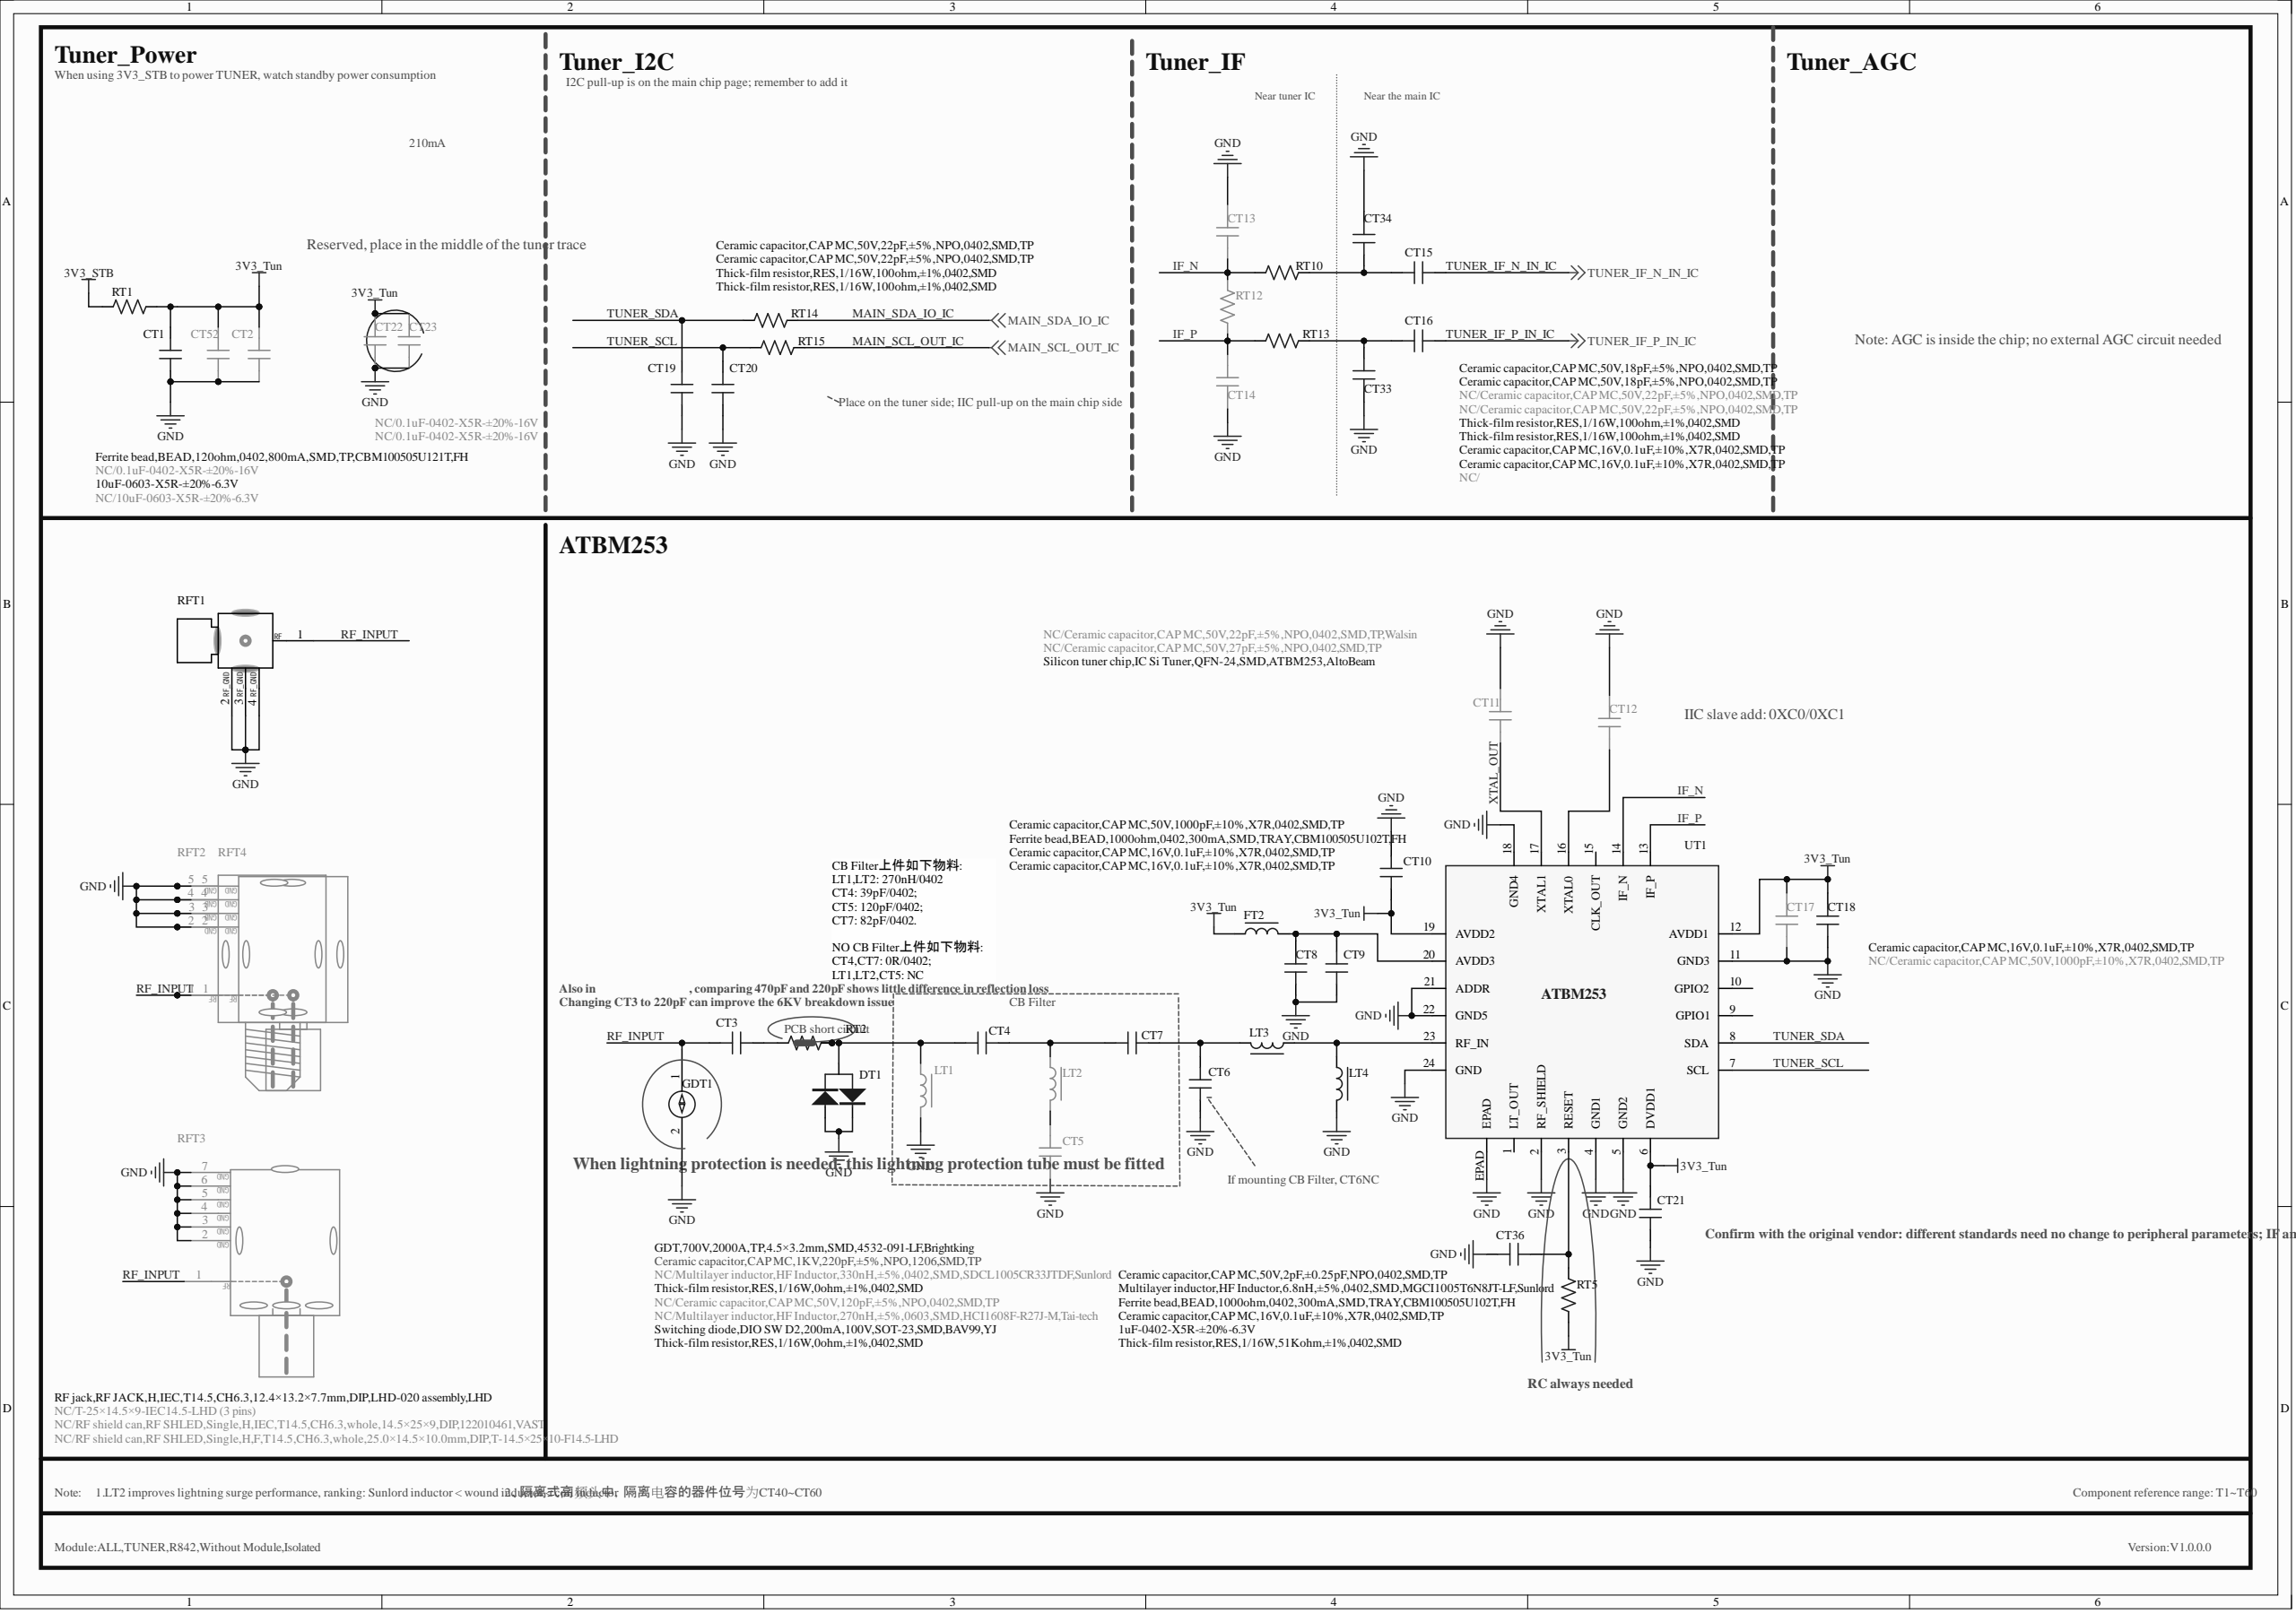Circuit board | Altium Designer | 527 parts | 243 nets | one sheet of the schematic
Parts on this sheet (reference | value | footprint):
CT1 | 10uF-0603-X5R-±20%-6.3V | C0603
CT2 | NC/0.1uF-0402-X5R-±20%-16V | C0402
CT3 | Ceramic capacitor,CAP MC,1KV,220pF,±5%,NPO,1206,SMD,TP | C1206
CT4 | Thick-film resistor,RES,1/16W,0ohm,±1%,0402,SMD | C0402
CT5 | NC/Ceramic capacitor,CAP MC,50V,120pF,±5%,NPO,0402,SMD,TP | C0402
CT6 | Ceramic capacitor,CAP MC,50V,2pF,±0.25pF,NPO,0402,SMD,TP | C0402
CT7 | Thick-film resistor,RES,1/16W,0ohm,±1%,0402,SMD | C0402
CT8 | Ceramic capacitor,CAP MC,16V,0.1uF,±10%,X7R,0402,SMD,TP | C0402
CT9 | Ceramic capacitor,CAP MC,50V,1000pF,±10%,X7R,0402,SMD,TP | C0402
CT10 | Ceramic capacitor,CAP MC,16V,0.1uF,±10%,X7R,0402,SMD,TP | C0402
CT11 | NC/Ceramic capacitor,CAP MC,50V,22pF,±5%,NPO,0402,SMD,TP,Walsin | C0402
CT12 | NC/Ceramic capacitor,CAP MC,50V,27pF,±5%,NPO,0402,SMD,TP | C0402
CT13 | NC/Ceramic capacitor,CAP MC,50V,22pF,±5%,NPO,0402,SMD,TP | C0402
CT14 | NC/Ceramic capacitor,CAP MC,50V,22pF,±5%,NPO,0402,SMD,TP | C0402
CT15 | Ceramic capacitor,CAP MC,16V,0.1uF,±10%,X7R,0402,SMD,TP | C0402
CT16 | Ceramic capacitor,CAP MC,16V,0.1uF,±10%,X7R,0402,SMD,TP | C0402
CT17 | NC/Ceramic capacitor,CAP MC,50V,1000pF,±10%,X7R,0402,SMD,TP | C0402
CT18 | Ceramic capacitor,CAP MC,16V,0.1uF,±10%,X7R,0402,SMD,TP | C0402
CT19 | Ceramic capacitor,CAP MC,50V,22pF,±5%,NPO,0402,SMD,TP | C0402
CT20 | Ceramic capacitor,CAP MC,50V,22pF,±5%,NPO,0402,SMD,TP | C0402
CT21 | Ceramic capacitor,CAP MC,16V,0.1uF,±10%,X7R,0402,SMD,TP | C0402
CT22 | NC/0.1uF-0402-X5R-±20%-16V | C0402
CT23 | NC/0.1uF-0402-X5R-±20%-16V | C0402
CT33 | Ceramic capacitor,CAP MC,50V,18pF,±5%,NPO,0402,SMD,TP | C0402
CT34 | Ceramic capacitor,CAP MC,50V,18pF,±5%,NPO,0402,SMD,TP | C0402
CT36 | 1uF-0402-X5R-±20%-6.3V | C0402
CT52 | NC/10uF-0603-X5R-±20%-6.3V | C0603
DT1 | Switching diode,DIO SW D2,200mA,100V,SOT-23,SMD,BAV99,YJ | SO-23
FT2 | Ferrite bead,BEAD,1000ohm,0402,300mA,SMD,TRAY,CBM100505U102T,FH | L0402
GDT1 | GDT,700V,2000A,TP,4.5×3.2mm,SMD,4532-091-LF,Brightking | SMD4532-1
LT1 | NC/Multilayer inductor,HF Inductor,330nH,±5%,0402,SMD,SDCL1005CR33JTDF,Sunlord | L0402
LT2 | NC/Multilayer inductor,HF Inductor,270nH,±5%,0603,SMD,HCI1608F-R27J-M,Tai-tech | L0603
LT3 | Multilayer inductor,HF Inductor,6.8nH,±5%,0402,SMD,MGCI1005T6N8JT-LF,Sunlord | L0402
LT4 | Ferrite bead,BEAD,1000ohm,0402,300mA,SMD,TRAY,CBM100505U102T,FH | L0402
RFT1 | RF jack,RF JACK,H,IEC,T14.5,CH6.3,12.4×13.2×7.7mm,DIP,LHD-020 assembly,LHD | ANT-IEC14.5-H-4
RFT2 | NC/RF shield can,RF SHLED,Single,H,IEC,T14.5,CH6.3,whole,14.5×25×9,DIP,122010461,VAST | T-14.5×25×9.0-IEC14.5
RFT3 | NC/T-25×14.5×9-IEC14.5-LHD (3 pins) | T-25×14.5×9-IEC14.5-LHD-1
RFT4 | NC/RF shield can,RF SHLED,Single,H,F,T14.5,CH6.3,whole,25.0×14.5×10.0mm,DIP,T-14.5×25×10-F14.5-LHD | T-14.5×25×10-F14.5
RT5 | Thick-film resistor,RES,1/16W,51Kohm,±1%,0402,SMD | R0402
RT10 | Thick-film resistor,RES,1/16W,100ohm,±1%,0402,SMD | R0402
RT12 | NC/ | R0402
RT13 | Thick-film resistor,RES,1/16W,100ohm,±1%,0402,SMD | R0402
RT14 | Thick-film resistor,RES,1/16W,100ohm,±1%,0402,SMD | R0402
RT15 | Thick-film resistor,RES,1/16W,100ohm,±1%,0402,SMD | R0402
UT1 | Silicon tuner chip,IC Si Tuner,QFN-24,SMD,ATBM253,AltoBeam | QFN24/0.4-1
Nets of these parts (net: part-pin ...):
XTAL_OUT: CT11-2 UT1-17
TUNER_SDA: CT19-2 RT14-1 UT1-8
TUNER_SCL: CT20-2 RT15-1 UT1-7
TUNER_IF_P_IN_IC: CT16-1
TUNER_IF_N_IN_IC: CT15-2
RF_INPUT: CT3-2 GDT1-1 RFT1-1 RFT2-1 RFT3-1 RFT4-1
NetLT3_2: LT3-2 LT4-2 UT1-23
NetCT36_1: CT36-1 RT5-2 UT1-3
NetCT16_2: CT16-2 CT33-2 RT13-2
NetCT15_1: CT15-1 CT34-1 RT10-2
NetCT12_2: CT12-2 UT1-16
NetCT8_1: CT8-1 CT9-2 FT2-1 UT1-20
NetCT6_1: CT6-1 CT7-1 LT3-1
NetCT5_1: CT5-1 LT2-2
NetCT4_2: CT4-2 DT1-2 LT1-2
NetCT4_1: CT4-1 CT7-2 LT2-1
NetCT3_1: CT3-1
MAIN_SDA_IO_IC: RT14-2
MAIN_SCL_OUT_IC: RT15-2
IF_P: CT14-2 RT12-1 RT13-1 UT1-13
IF_N: CT13-1 RT10-1 RT12-2 UT1-14
GND: CT1-1 CT2-1 CT5-2 CT6-2 CT8-2 CT9-1 CT10-1 CT11-1 CT12-1 CT13-2 CT14-1 CT17-2 CT18-1 CT19-1 CT20-1 CT21-1 CT22-2 CT23-2 CT33-1 CT34-2 CT36-2 CT52-1 DT1-1 DT1-3 GDT1-2 LT1-1 LT4-1 RFT1-2 RFT1-3 RFT1-4 RFT2-2 RFT2-3 RFT2-4 RFT2-5 RFT3-2 RFT3-3 RFT3-4 RFT3-5 RFT3-6 RFT3-7 RFT4-2 RFT4-3 RFT4-4 RFT4-5 UT1-2 UT1-4 UT1-5 UT1-11 UT1-18 UT1-21 UT1-22 UT1-24 UT1-EPAD
3V3_Tun: CT1-2 CT2-2 CT10-2 CT17-1 CT18-2 CT21-2 CT22-1 CT23-1 CT52-2 FT2-2 RT5-1 UT1-6 UT1-12 UT1-19